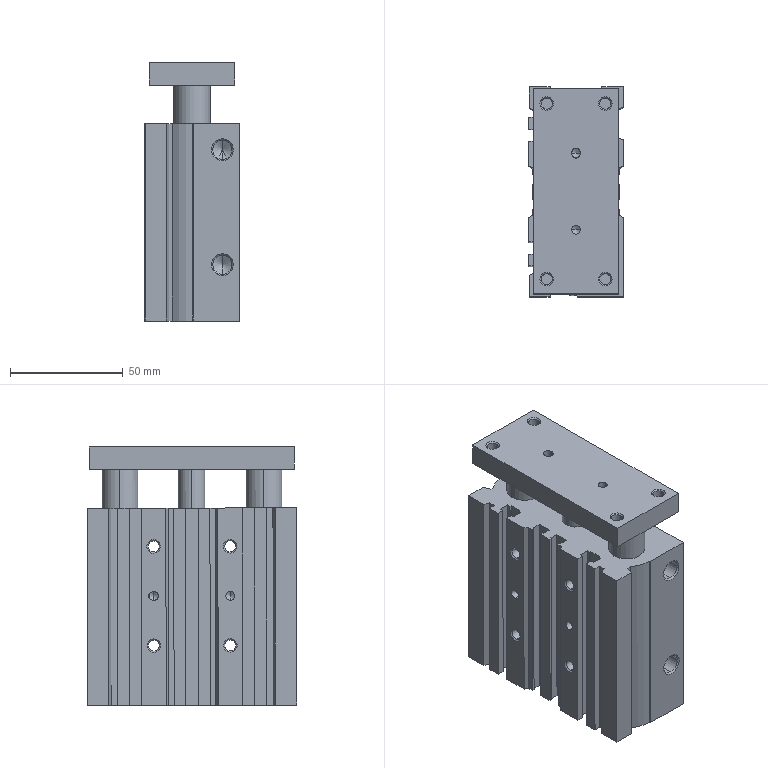Part | SolidWorks | 2 solids | 271 faces | box 42 x 93.165 x 114.867 mm | volume 308752 mm3 | plane 127 | cylinder 84 | cone 60 | commonest cylinder face diameters 4.917 x24 4 x18 5.4 x8 8.566 x8 9.5 x8 16 x8